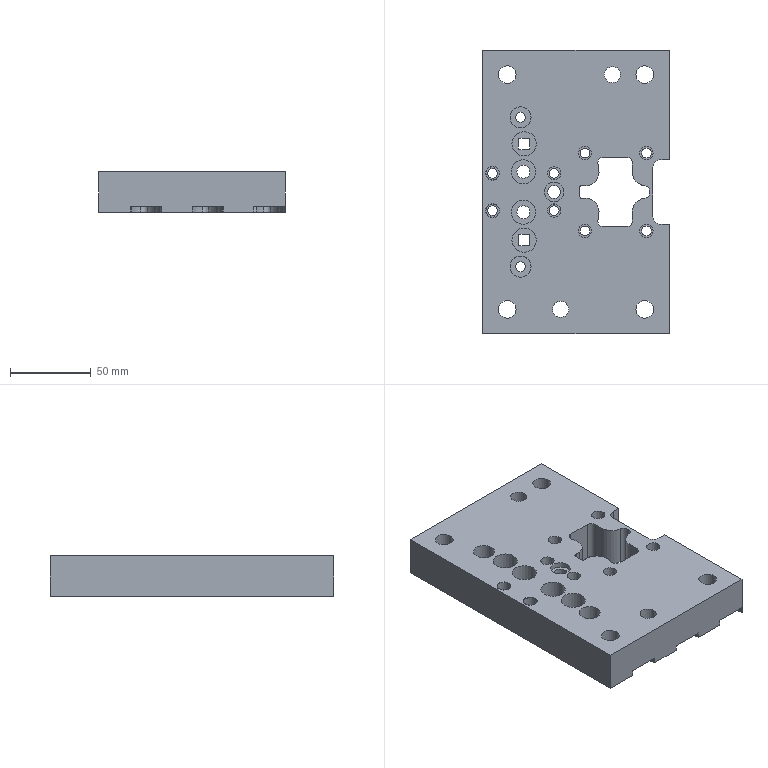Part | STEP file | PN_0039_id846_x_t | 1 solid | 211 faces | box 115 x 175 x 25 mm | volume 409284 mm3 | spline 76 | cylinder 76 | plane 59 | commonest cylinder face diameters 6 x14 2 x8 8.2 x8 7 x6 14.536 x6 10 x4